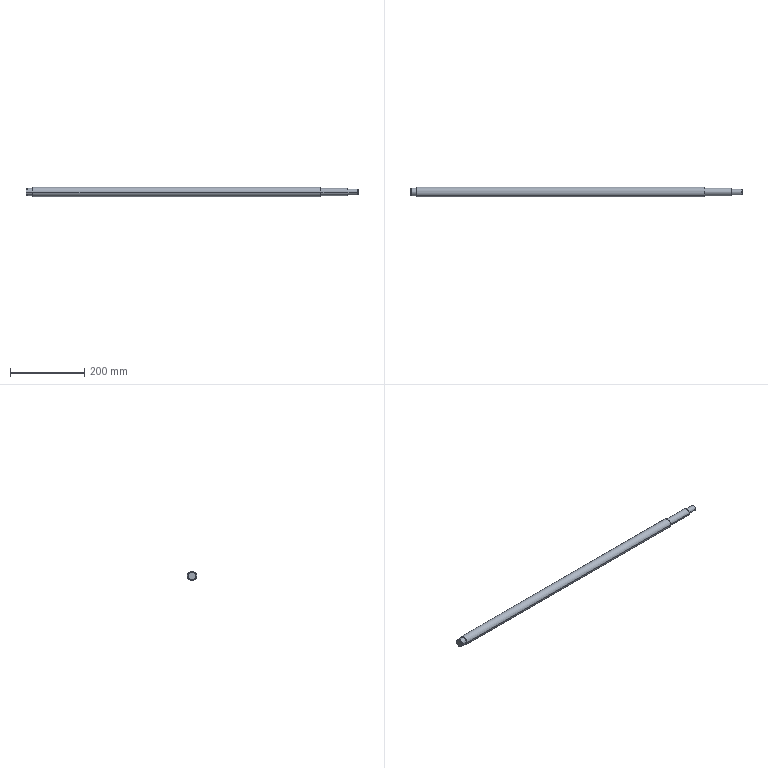Part | STEP file | 0244_Z_001_BSST2510-1195_1 | 1 solid | 29 faces | box 895 x 25 x 25 mm | volume 414687 mm3 | cylinder 12 | cone 10 | plane 7 | commonest cylinder face diameters 20 x6 15 x2 19 x2 25 x2